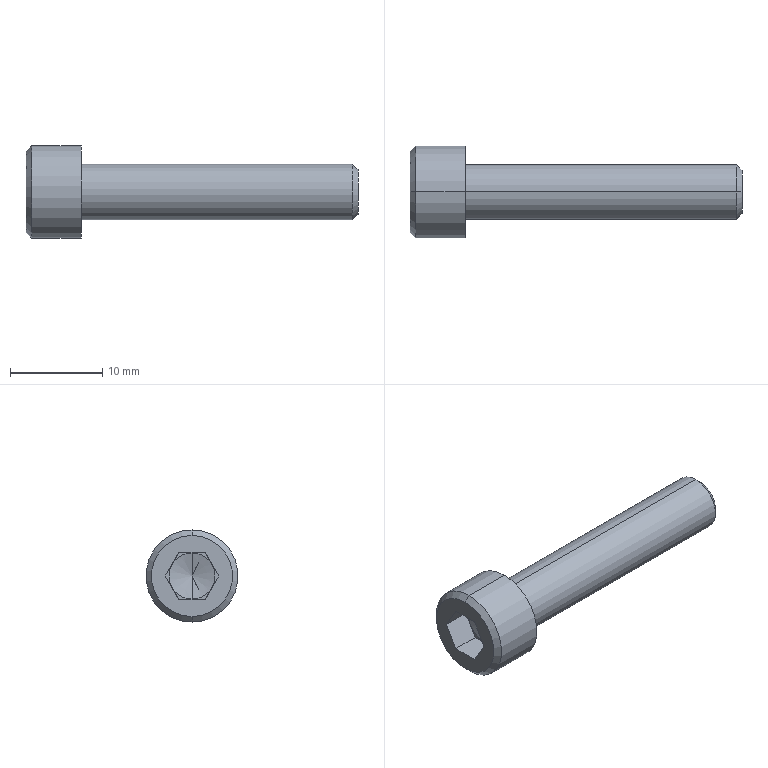Part | STEP file | ASCB6-30 | 1 solid | 25 faces | box 36 x 10 x 10 mm | volume 1241 mm3 | plane 15 | cone 6 | cylinder 4 | commonest cylinder face diameters 6 x2 10 x2